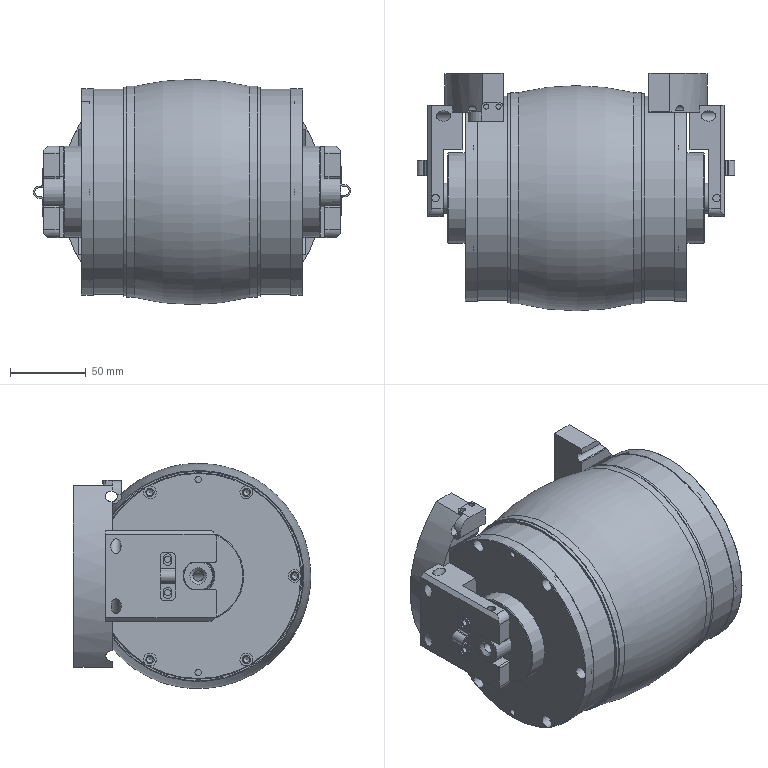Part | NX | features BREP 30 | 61 solids | 2306 faces | box 209 x 156.238 x 148.156 mm | volume 1731844 mm3 | cylinder 1267 | plane 609 | cone 169 | torus 159 | sphere 66 | spline 36 | commonest cylinder face diameters 12 x255 26.248 x120 3 x84 7.2 x72 33 x61 32.998 x60